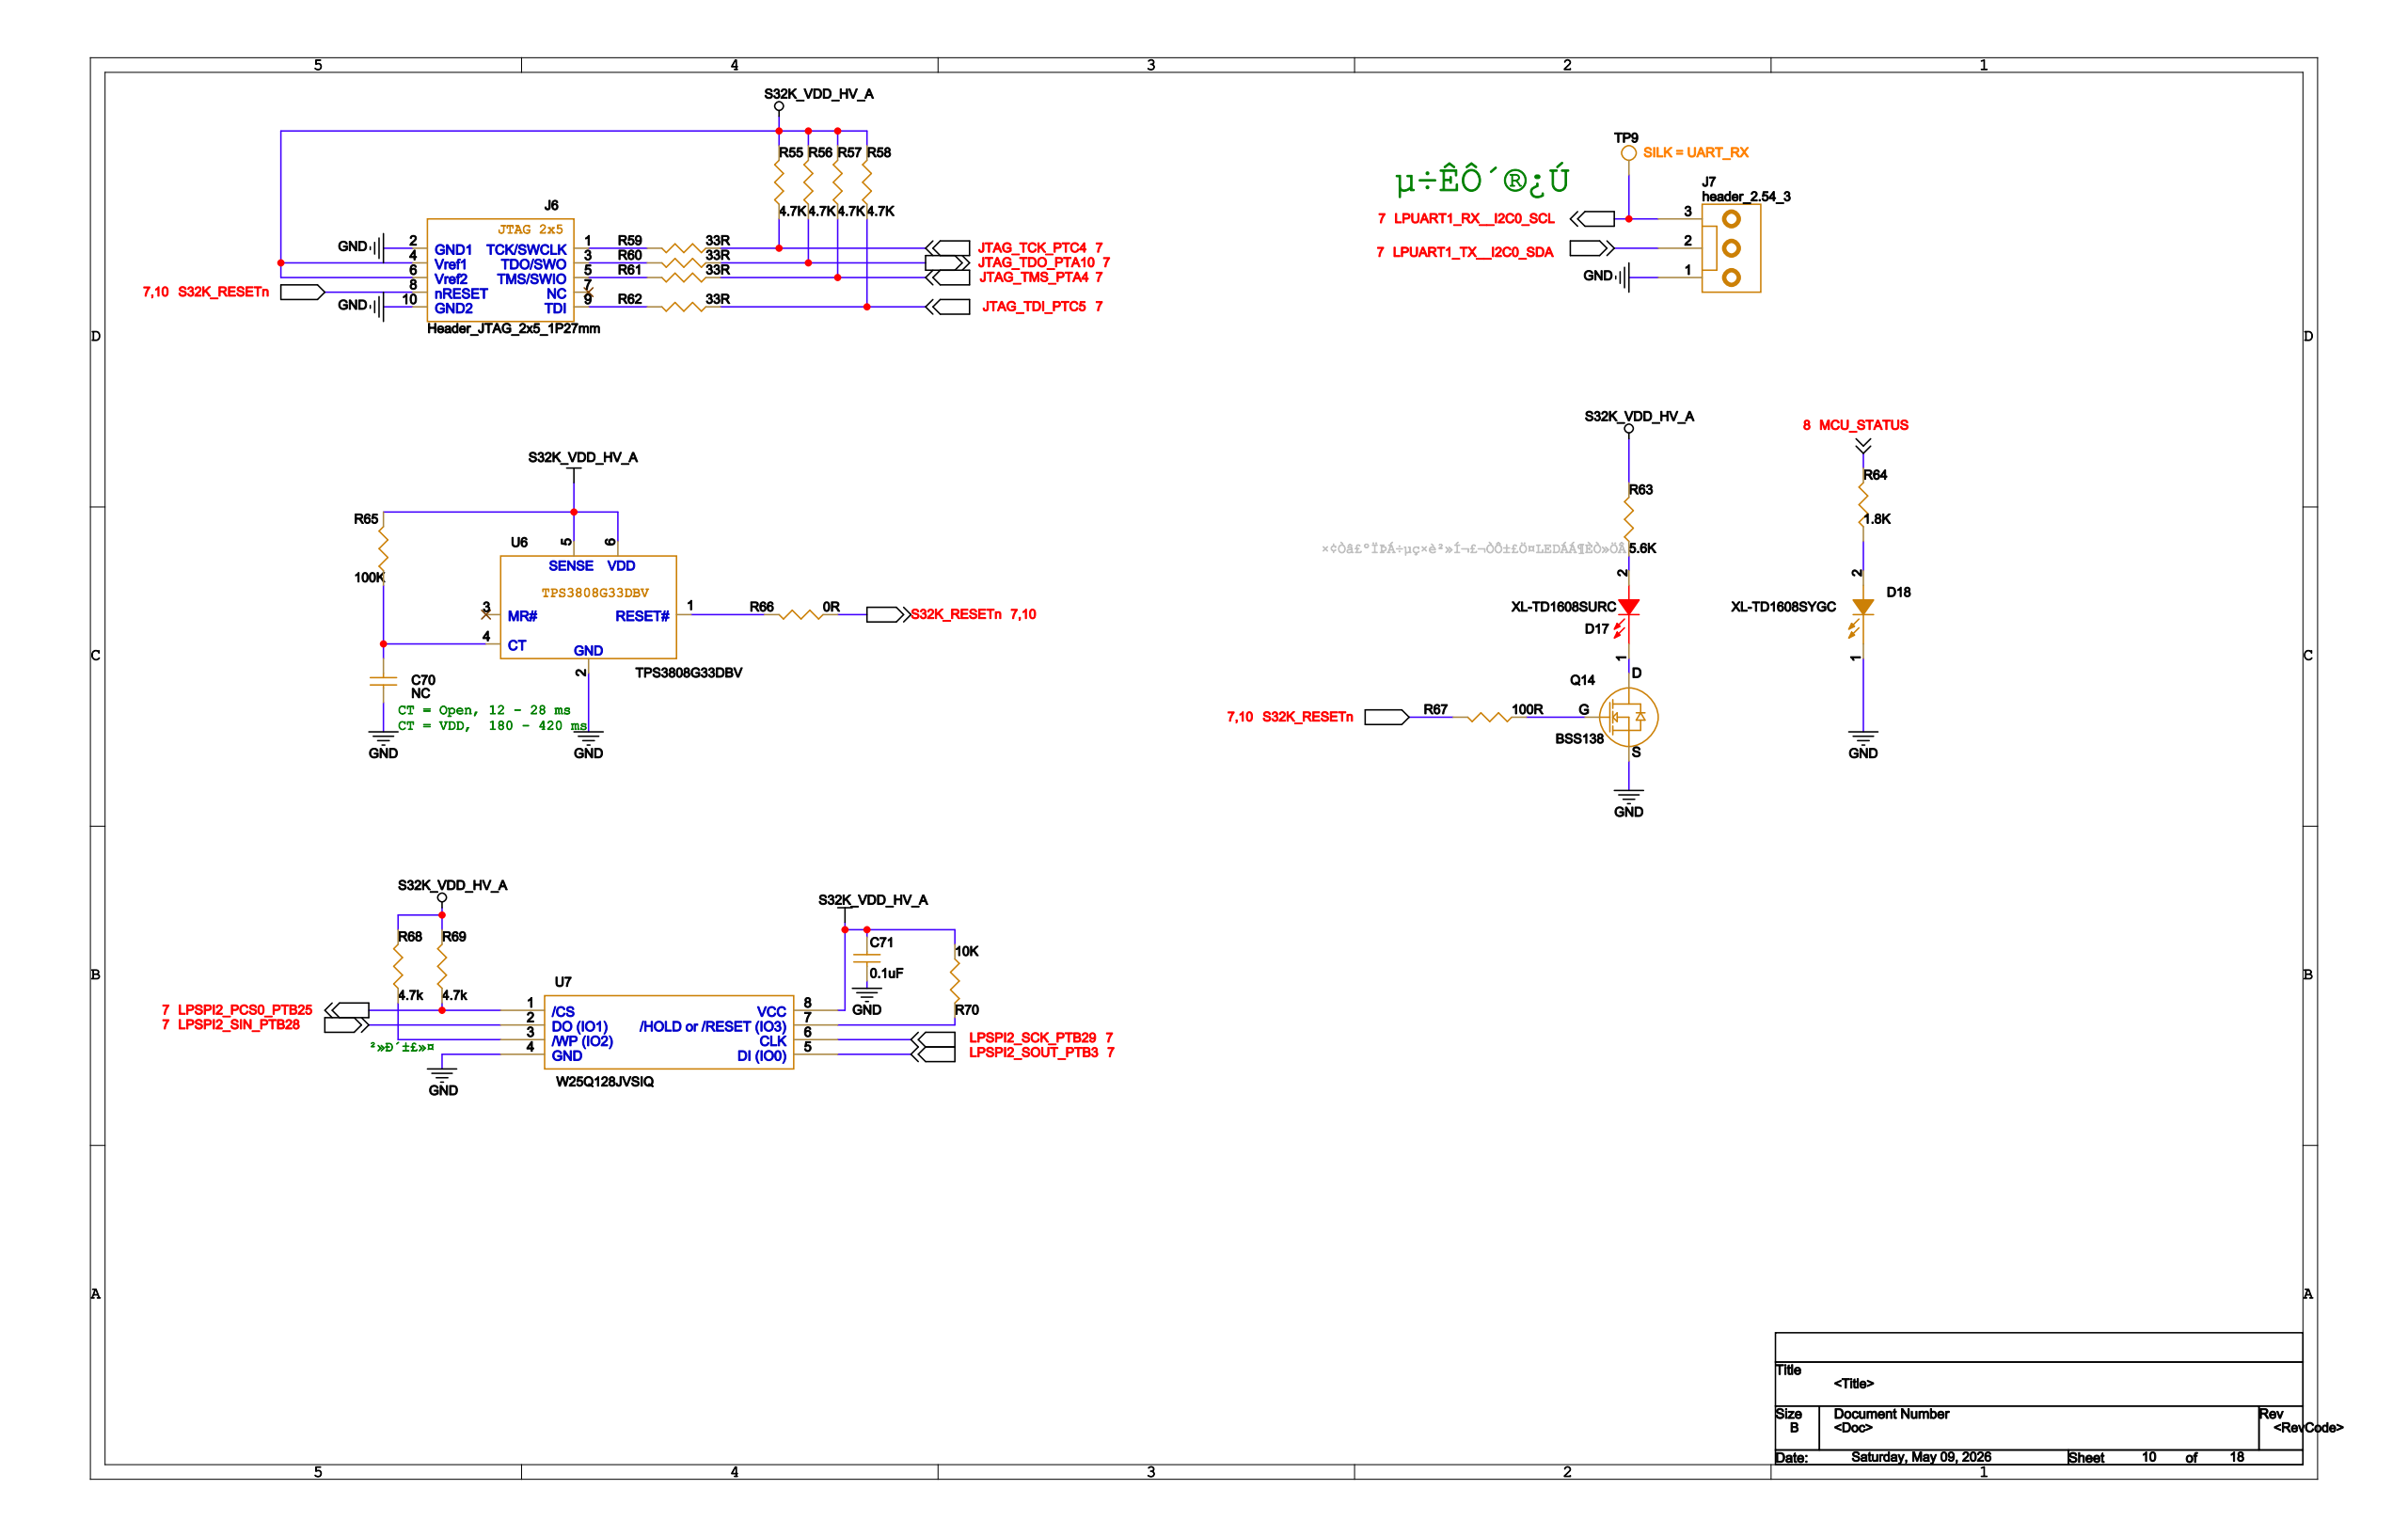Circuit board | Cadence Allegro | 330 parts | 215 nets | one sheet of the schematic
Parts on this sheet (reference | value | footprint):
C70 | NC | 0402
C71 | 0.1uF | 0402
D17 | XL-TD1608SURC | LED0603
D18 | XL-TD1608SYGC | LED0603
J6 | Header_JTAG_2x5_1P27mm | JTAG_2X5_1P27MM
J7 | header_2.54_3 | HDR_1X3
Q14 | BSS138 | 003_SOT23B
R55 | 4.7K | 0402
R56 | 4.7K | 0402
R57 | 4.7K | 0402
R58 | 4.7K | 0402
R59 | 33R | 0402
R60 | 33R | 0402
R61 | 33R | 0402
R62 | 33R | 0402
R63 | 5.6K | 0402
R64 | 1.8K | 0402
R65 | 100K | 0402
R66 | 0R | 0402
R67 | 100R | 0402
R68 | 4.7K | 0402
R69 | 4.7K | 0402
R70 | 10K | 0402
TP9 | TP | S0400CI
U6 | TPS3808G33DBV | SOT23_6P_29X28_H150
U7 | W25Q128JVSIQ | SO8P_79_127_H220
Nets of these parts (net: part-pin ...):
GND: C70-1 C71-2 D18-1 J6-2 J6-10 J7-1 Q14-S U6-2 U7-4
S32K_VDD_HV_A: C71-1 J6-4 J6-6 R55-2 R56-2 R57-2 R58-2 R63-2 R65-2 R68-1 R69-1 R70-2 U6-5 U6-6 U7-8
N16956186: C70-2 R65-1 U6-4
N16781545: D17-1 Q14-D
N2187762: D17-2 R63-1
N16903536: D18-2 R64-1
S32K_RESETN: J6-8 R66-1 R67-2
N1674196: J6-1 R59-1
N1674346: J6-9 R62-1
N1674242: J6-3 R60-1
N1674294: J6-5 R61-1
LPUART1_TX__I2C0_SDA: J7-2
LPUART1_RX__I2C0_SCL: J7-3 TP9-1
JTAG_TCK_PTC4: R55-1 R59-2
JTAG_TDO_PTA10: R56-1 R60-2
JTAG_TMS_PTA4: R57-1 R61-2
JTAG_TDI_PTC5: R58-1 R62-2
N2523682: R68-2 U7-3
LPSPI2_PCS0_PTB25: R69-2 U7-1
MCU_STATUS: R64-2
N16956201: R66-2 U6-1
N1972160: R70-1 U7-7
N2188456: Q14-G R67-1
LPSPI2_SIN_PTB28: U7-2
LPSPI2_SCK_PTB29: U7-6
LPSPI2_SOUT_PTB3: U7-5